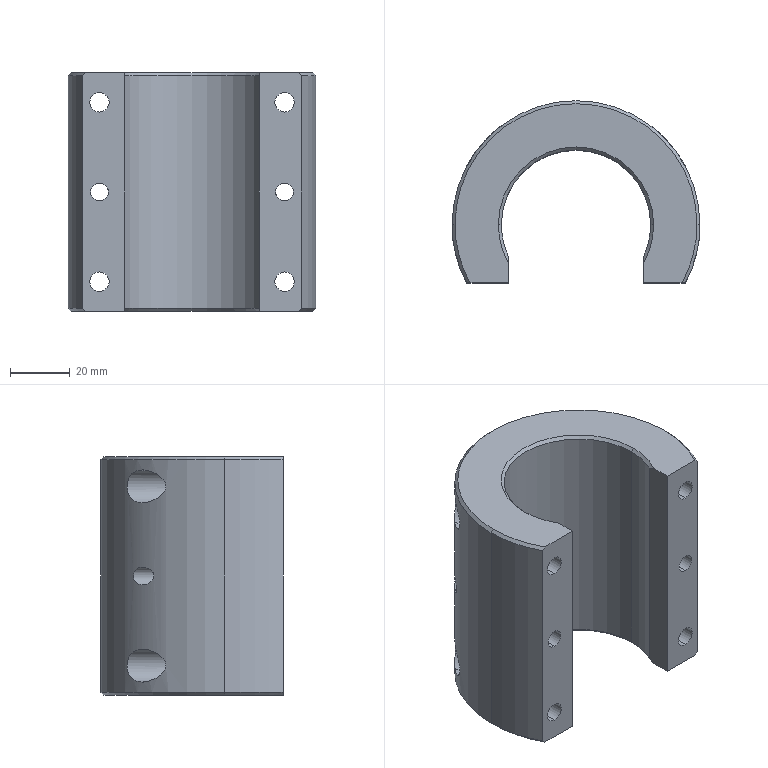Part | STEP file | PN_0042 | 1 solid | 48 faces | box 83 x 61 x 80 mm | volume 174767 mm3 | cylinder 26 | cone 12 | plane 10 | commonest cylinder face diameters 6.5 x8 11 x8 6 x4 50 x3 83 x3